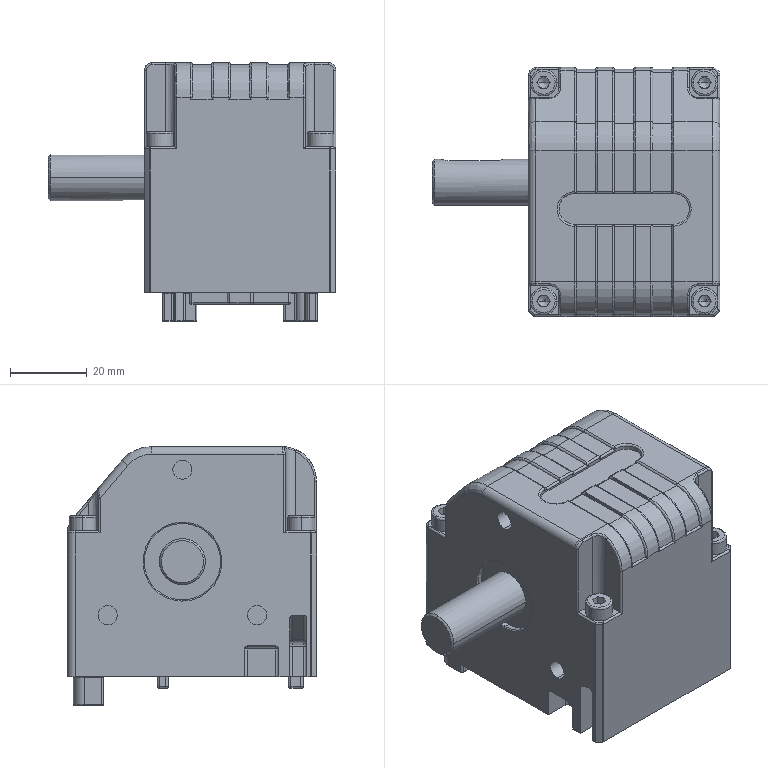Part | STEP file | Copy of K50-right output shaft^K50A-1H20-S(formula driven)-L300-motor left- | 7 solids | 718 faces | box 75.1 x 65 x 67.5 mm | volume 175546 mm3 | cylinder 295 | plane 209 | spline 188 | cone 26 | commonest cylinder face diameters 1 x85 5 x38 0.4 x24 4 x22 1.6 x18 0.6 x12